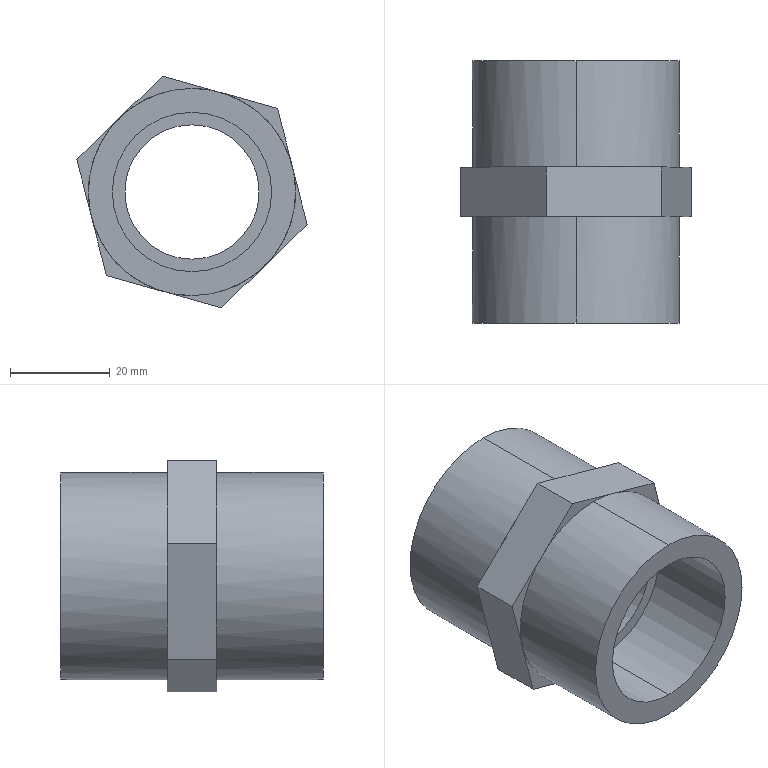Part | SolidWorks | features ICE 3, Revolution 2 | 1 solid | 34 faces | box 46.249 x 52.7 x 46.542 mm | volume 34114 mm3 | plane 22 | cylinder 10 | cone 2 | commonest cylinder face diameters 32 x4 41.6 x4 27 x2
STEP:
#1=CARTESIAN_POINT('',(0.,7.5,-13.5));
#2=VERTEX_POINT('',#1);
#3=CARTESIAN_POINT('',(0.,7.5,13.5));
#4=VERTEX_POINT('',#3);
#5=CARTESIAN_POINT('',(0.,7.5,0.));
#6=DIRECTION('',(0.,1.,0.));
#7=DIRECTION('',(0.,0.,1.));
#8=AXIS2_PLACEMENT_3D('',#5,#6,#7);
#9=CIRCLE('',#8,13.5);
#10=EDGE_CURVE('',#2,#4,#9,.T.);
#11=ORIENTED_EDGE('',*,*,#10,.T.);
#12=CARTESIAN_POINT('',(0.,-7.5,13.5));
#13=VERTEX_POINT('',#12);
#14=CARTESIAN_POINT('',(0.,7.5,13.5));
#15=DIRECTION('',(0.,-1.,0.));
#16=VECTOR('',#15,1000.);
#17=LINE('',#14,#16);
#18=EDGE_CURVE('',#4,#13,#17,.T.);
#19=ORIENTED_EDGE('',*,*,#18,.T.);
#20=CARTESIAN_POINT('',(0.,-7.5,-13.5));
#21=VERTEX_POINT('',#20);
#22=CARTESIAN_POINT('',(0.,-7.5,0.));
#23=DIRECTION('',(0.,1.,0.));
#24=DIRECTION('',(0.,0.,1.));
#25=AXIS2_PLACEMENT_3D('',#22,#23,#24);
#26=CIRCLE('',#25,13.5);
#27=EDGE_CURVE('',#21,#13,#26,.T.);
#28=ORIENTED_EDGE('',*,*,#27,.F.);
#29=CARTESIAN_POINT('',(0.,7.5,-13.5));
#30=DIRECTION('',(0.,-1.,0.));
#31=VECTOR('',#30,1000.);
#32=LINE('',#29,#31);
#33=EDGE_CURVE('',#2,#21,#32,.T.);
#34=ORIENTED_EDGE('',*,*,#33,.F.);
#35=EDGE_LOOP('',(#11,#19,#28,#34));
#36=FACE_OUTER_BOUND('',#35,.T.);
#37=CARTESIAN_POINT('',(0.,7.5,0.));
#38=DIRECTION('',(0.,-1.,0.));
#39=DIRECTION('',(0.,0.,-1.));
#40=AXIS2_PLACEMENT_3D('',#37,#38,#39);
#41=CYLINDRICAL_SURFACE('',#40,13.5);
#42=ADVANCED_FACE('',(#36),#41,.F.);
#43=CARTESIAN_POINT('',(0.,26.2,16.));
#44=VERTEX_POINT('',#43);
#45=CARTESIAN_POINT('',(0.,26.2,-16.));
#46=VERTEX_POINT('',#45);
#47=CARTESIAN_POINT('',(0.,26.2,0.));
#48=DIRECTION('',(0.,-1.,0.));
#49=DIRECTION('',(0.,0.,-1.));
#50=AXIS2_PLACEMENT_3D('',#47,#48,#49);
#51=CIRCLE('',#50,16.);
#52=EDGE_CURVE('',#44,#46,#51,.T.);
#53=ORIENTED_EDGE('',*,*,#52,.T.);
#54=CARTESIAN_POINT('',(0.,26.35,-16.15));
#55=VERTEX_POINT('',#54);
#56=CARTESIAN_POINT('',(0.,26.2,-16.));
#57=DIRECTION('',(0.,0.7071,-0.7071));
#58=VECTOR('',#57,1000.);
#59=LINE('',#56,#58);
#60=EDGE_CURVE('',#46,#55,#59,.T.);
#61=ORIENTED_EDGE('',*,*,#60,.T.);
#62=CARTESIAN_POINT('',(0.,26.35,16.15));
#63=VERTEX_POINT('',#62);
#64=CARTESIAN_POINT('',(0.,26.35,0.));
#65=DIRECTION('',(0.,-1.,0.));
#66=DIRECTION('',(0.,0.,-1.));
#67=AXIS2_PLACEMENT_3D('',#64,#65,#66);
#68=CIRCLE('',#67,16.15);
#69=EDGE_CURVE('',#63,#55,#68,.T.);
#70=ORIENTED_EDGE('',*,*,#69,.F.);
#71=CARTESIAN_POINT('',(0.,26.2,16.));
#72=DIRECTION('',(0.,0.7071,0.7071));
#73=VECTOR('',#72,1000.);
#74=LINE('',#71,#73);
#75=EDGE_CURVE('',#44,#63,#74,.T.);
#76=ORIENTED_EDGE('',*,*,#75,.F.);
#77=EDGE_LOOP('',(#53,#61,#70,#76));
#78=FACE_OUTER_BOUND('',#77,.T.);
#79=CARTESIAN_POINT('',(0.,26.2,0.));
#80=DIRECTION('',(0.,1.,0.));
#81=DIRECTION('',(0.,0.,1.));
#82=AXIS2_PLACEMENT_3D('',#79,#80,#81);
#83=CONICAL_SURFACE('',#82,16.,0.7854);
#84=ADVANCED_FACE('',(#78),#83,.F.);
#85=CARTESIAN_POINT('',(0.,26.35,-20.8));
#86=VERTEX_POINT('',#85);
#87=CARTESIAN_POINT('',(0.,26.35,20.8));
#88=VERTEX_POINT('',#87);
#89=CARTESIAN_POINT('',(0.,26.35,0.));
#90=DIRECTION('',(0.,-1.,0.));
#91=DIRECTION('',(0.,0.,-1.));
#92=AXIS2_PLACEMENT_3D('',#89,#90,#91);
#93=CIRCLE('',#92,20.8);
#94=EDGE_CURVE('',#86,#88,#93,.T.);
#95=ORIENTED_EDGE('',*,*,#94,.T.);
#96=CARTESIAN_POINT('',(0.,5.,20.8));
#97=VERTEX_POINT('',#96);
#98=CARTESIAN_POINT('',(0.,-26.35,20.8));
#99=DIRECTION('',(0.,-1.,0.));
#100=VECTOR('',#99,1000.);
#101=LINE('',#98,#100);
#102=EDGE_CURVE('',#88,#97,#101,.T.);
#103=ORIENTED_EDGE('',*,*,#102,.T.);
#104=CARTESIAN_POINT('',(5.62,5.,20.026));
#105=VERTEX_POINT('',#104);
#106=CARTESIAN_POINT('',(0.,5.,0.));
#107=DIRECTION('',(0.,1.,0.));
#108=DIRECTION('',(0.,0.,1.));
#109=AXIS2_PLACEMENT_3D('',#106,#107,#108);
#110=CIRCLE('',#109,20.8);
#111=EDGE_CURVE('',#97,#105,#110,.T.);
#112=ORIENTED_EDGE('',*,*,#111,.T.);
#113=CARTESIAN_POINT('',(20.153,5.,5.146));
#114=VERTEX_POINT('',#113);
#115=CARTESIAN_POINT('',(0.,5.,0.));
#116=DIRECTION('',(0.,1.,0.));
#117=DIRECTION('',(0.,0.,1.));
#118=AXIS2_PLACEMENT_3D('',#115,#116,#117);
#119=CIRCLE('',#118,20.8);
#120=EDGE_CURVE('',#105,#114,#119,.T.);
#121=ORIENTED_EDGE('',*,*,#120,.T.);
#122=CARTESIAN_POINT('',(14.533,5.,-14.88));
#123=VERTEX_POINT('',#122);
#124=CARTESIAN_POINT('',(0.,5.,0.));
#125=DIRECTION('',(0.,1.,0.));
#126=DIRECTION('',(0.,0.,1.));
#127=AXIS2_PLACEMENT_3D('',#124,#125,#126);
#128=CIRCLE('',#127,20.8);
#129=EDGE_CURVE('',#114,#123,#128,.T.);
#130=ORIENTED_EDGE('',*,*,#129,.T.);
#131=CARTESIAN_POINT('',(0.,5.,-20.8));
#132=VERTEX_POINT('',#131);
#133=CARTESIAN_POINT('',(0.,5.,0.));
#134=DIRECTION('',(0.,1.,0.));
#135=DIRECTION('',(0.,0.,1.));
#136=AXIS2_PLACEMENT_3D('',#133,#134,#135);
#137=CIRCLE('',#136,20.8);
#138=EDGE_CURVE('',#123,#132,#137,.T.);
#139=ORIENTED_EDGE('',*,*,#138,.T.);
#140=CARTESIAN_POINT('',(0.,-26.35,-20.8));
#141=DIRECTION('',(0.,-1.,0.));
#142=VECTOR('',#141,1000.);
#143=LINE('',#140,#142);
#144=EDGE_CURVE('',#86,#132,#143,.T.);
#145=ORIENTED_EDGE('',*,*,#144,.F.);
#146=EDGE_LOOP('',(#95,#103,#112,#121,#130,#139,#145));
#147=FACE_OUTER_BOUND('',#146,.T.);
#148=CARTESIAN_POINT('',(0.,-26.35,0.));
#149=DIRECTION('',(0.,-1.,0.));
#150=DIRECTION('',(0.,0.,-1.));
#151=AXIS2_PLACEMENT_3D('',#148,#149,#150);
#152=CYLINDRICAL_SURFACE('',#151,20.8);
#153=ADVANCED_FACE('',(#147),#152,.T.);
#154=ORIENTED_EDGE('',*,*,#52,.F.);
#155=CARTESIAN_POINT('',(0.,7.5,16.));
#156=VERTEX_POINT('',#155);
#157=CARTESIAN_POINT('',(0.,-26.35,16.));
#158=DIRECTION('',(0.,-1.,0.));
#159=VECTOR('',#158,1000.);
#160=LINE('',#157,#159);
#161=EDGE_CURVE('',#44,#156,#160,.T.);
#162=ORIENTED_EDGE('',*,*,#161,.T.);
#163=CARTESIAN_POINT('',(0.,7.5,-16.));
#164=VERTEX_POINT('',#163);
#165=CARTESIAN_POINT('',(0.,7.5,0.));
#166=DIRECTION('',(0.,-1.,0.));
#167=DIRECTION('',(0.,0.,1.));
#168=AXIS2_PLACEMENT_3D('',#165,#166,#167);
#169=CIRCLE('',#168,16.);
#170=EDGE_CURVE('',#156,#164,#169,.T.);
#171=ORIENTED_EDGE('',*,*,#170,.T.);
#172=CARTESIAN_POINT('',(0.,-26.35,-16.));
#173=DIRECTION('',(0.,-1.,0.));
#174=VECTOR('',#173,1000.);
#175=LINE('',#172,#174);
#176=EDGE_CURVE('',#46,#164,#175,.T.);
#177=ORIENTED_EDGE('',*,*,#176,.F.);
#178=EDGE_LOOP('',(#154,#162,#171,#177));
#179=FACE_OUTER_BOUND('',#178,.T.);
#180=CARTESIAN_POINT('',(0.,-26.35,0.));
#181=DIRECTION('',(0.,-1.,0.));
#182=DIRECTION('',(0.,0.,-1.));
#183=AXIS2_PLACEMENT_3D('',#180,#181,#182);
#184=CYLINDRICAL_SURFACE('',#183,16.);
#185=ADVANCED_FACE('',(#179),#184,.F.);
#186=CARTESIAN_POINT('',(0.,-5.,20.8));
#187=VERTEX_POINT('',#186);
#188=CARTESIAN_POINT('',(5.62,-5.,20.026));
#189=VERTEX_POINT('',#188);
#190=CARTESIAN_POINT('',(0.,-5.,0.));
#191=DIRECTION('',(0.,1.,0.));
#192=DIRECTION('',(0.,0.,1.));
#193=AXIS2_PLACEMENT_3D('',#190,#191,#192);
#194=CIRCLE('',#193,20.8);
#195=EDGE_CURVE('',#187,#189,#194,.T.);
#196=ORIENTED_EDGE('',*,*,#195,.F.);
#197=CARTESIAN_POINT('',(0.,-26.35,20.8));
#198=VERTEX_POINT('',#197);
#199=CARTESIAN_POINT('',(0.,-26.35,20.8));
#200=DIRECTION('',(0.,-1.,0.));
#201=VECTOR('',#200,1000.);
#202=LINE('',#199,#201);
#203=EDGE_CURVE('',#187,#198,#202,.T.);
#204=ORIENTED_EDGE('',*,*,#203,.T.);
#205=CARTESIAN_POINT('',(0.,-26.35,-20.8));
#206=VERTEX_POINT('',#205);
#207=CARTESIAN_POINT('',(0.,-26.35,0.));
#208=DIRECTION('',(0.,-1.,0.));
#209=DIRECTION('',(0.,0.,-1.));
#210=AXIS2_PLACEMENT_3D('',#207,#208,#209);
#211=CIRCLE('',#210,20.8);
#212=EDGE_CURVE('',#206,#198,#211,.T.);
#213=ORIENTED_EDGE('',*,*,#212,.F.);
#214=CARTESIAN_POINT('',(0.,-5.,-20.8));
#215=VERTEX_POINT('',#214);
#216=CARTESIAN_POINT('',(0.,-26.35,-20.8));
#217=DIRECTION('',(0.,-1.,0.));
#218=VECTOR('',#217,1000.);
#219=LINE('',#216,#218);
#220=EDGE_CURVE('',#215,#206,#219,.T.);
#221=ORIENTED_EDGE('',*,*,#220,.F.);
#222=CARTESIAN_POINT('',(14.533,-5.,-14.88));
#223=VERTEX_POINT('',#222);
#224=CARTESIAN_POINT('',(0.,-5.,0.));
#225=DIRECTION('',(0.,1.,0.));
#226=DIRECTION('',(0.,0.,1.));
#227=AXIS2_PLACEMENT_3D('',#224,#225,#226);
#228=CIRCLE('',#227,20.8);
#229=EDGE_CURVE('',#223,#215,#228,.T.);
#230=ORIENTED_EDGE('',*,*,#229,.F.);
#231=CARTESIAN_POINT('',(20.153,-5.,5.146));
#232=VERTEX_POINT('',#231);
#233=CARTESIAN_POINT('',(0.,-5.,0.));
#234=DIRECTION('',(0.,1.,0.));
#235=DIRECTION('',(0.,0.,1.));
#236=AXIS2_PLACEMENT_3D('',#233,#234,#235);
#237=CIRCLE('',#236,20.8);
#238=EDGE_CURVE('',#232,#223,#237,.T.);
#239=ORIENTED_EDGE('',*,*,#238,.F.);
#240=CARTESIAN_POINT('',(0.,-5.,0.));
#241=DIRECTION('',(0.,1.,0.));
#242=DIRECTION('',(0.,0.,1.));
#243=AXIS2_PLACEMENT_3D('',#240,#241,#242);
#244=CIRCLE('',#243,20.8);
#245=EDGE_CURVE('',#189,#232,#244,.T.);
#246=ORIENTED_EDGE('',*,*,#245,.F.);
#247=EDGE_LOOP('',(#196,#204,#213,#221,#230,#239,#246));
#248=FACE_OUTER_BOUND('',#247,.T.);
#249=CARTESIAN_POINT('',(0.,-26.35,0.));
#250=DIRECTION('',(0.,-1.,0.));
#251=DIRECTION('',(0.,0.,-1.));
#252=AXIS2_PLACEMENT_3D('',#249,#250,#251);
#253=CYLINDRICAL_SURFACE('',#252,20.8);
#254=ADVANCED_FACE('',(#248),#253,.T.);
#255=CARTESIAN_POINT('',(0.,-7.5,16.));
#256=VERTEX_POINT('',#255);
#257=CARTESIAN_POINT('',(0.,-7.5,-16.));
#258=VERTEX_POINT('',#257);
#259=CARTESIAN_POINT('',(0.,-7.5,0.));
#260=DIRECTION('',(0.,-1.,0.));
#261=DIRECTION('',(0.,0.,1.));
#262=AXIS2_PLACEMENT_3D('',#259,#260,#261);
#263=CIRCLE('',#262,16.);
#264=EDGE_CURVE('',#256,#258,#263,.T.);
#265=ORIENTED_EDGE('',*,*,#264,.F.);
#266=CARTESIAN_POINT('',(0.,-26.35,16.));
#267=VERTEX_POINT('',#266);
#268=CARTESIAN_POINT('',(0.,-26.35,16.));
#269=DIRECTION('',(0.,-1.,0.));
#270=VECTOR('',#269,1000.);
#271=LINE('',#268,#270);
#272=EDGE_CURVE('',#256,#267,#271,.T.);
#273=ORIENTED_EDGE('',*,*,#272,.T.);
#274=CARTESIAN_POINT('',(0.,-26.35,-16.));
#275=VERTEX_POINT('',#274);
#276=CARTESIAN_POINT('',(0.,-26.35,0.));
#277=DIRECTION('',(0.,-1.,0.));
#278=DIRECTION('',(0.,0.,-1.));
#279=AXIS2_PLACEMENT_3D('',#276,#277,#278);
#280=CIRCLE('',#279,16.);
#281=EDGE_CURVE('',#267,#275,#280,.T.);
#282=ORIENTED_EDGE('',*,*,#281,.T.);
#283=CARTESIAN_POINT('',(0.,-26.35,-16.));
#284=DIRECTION('',(0.,-1.,0.));
#285=VECTOR('',#284,1000.);
#286=LINE('',#283,#285);
#287=EDGE_CURVE('',#258,#275,#286,.T.);
#288=ORIENTED_EDGE('',*,*,#287,.F.);
#289=EDGE_LOOP('',(#265,#273,#282,#288));
#290=FACE_OUTER_BOUND('',#289,.T.);
#291=CARTESIAN_POINT('',(0.,-26.35,0.));
#292=DIRECTION('',(0.,-1.,0.));
#293=DIRECTION('',(0.,0.,-1.));
#294=AXIS2_PLACEMENT_3D('',#291,#292,#293);
#295=CYLINDRICAL_SURFACE('',#294,16.);
#296=ADVANCED_FACE('',(#290),#295,.F.);
#297=ORIENTED_EDGE('',*,*,#272,.F.);
#298=CARTESIAN_POINT('',(0.,-7.5,0.));
#299=DIRECTION('',(0.,-1.,0.));
#300=DIRECTION('',(0.,0.,1.));
#301=AXIS2_PLACEMENT_3D('',#298,#299,#300);
#302=CIRCLE('',#301,16.);
#303=EDGE_CURVE('',#258,#256,#302,.T.);
#304=ORIENTED_EDGE('',*,*,#303,.F.);
#305=ORIENTED_EDGE('',*,*,#287,.T.);
#306=CARTESIAN_POINT('',(0.,-26.35,0.));
#307=DIRECTION('',(0.,-1.,0.));
#308=DIRECTION('',(0.,0.,-1.));
#309=AXIS2_PLACEMENT_3D('',#306,#307,#308);
#310=CIRCLE('',#309,16.);
#311=EDGE_CURVE('',#275,#267,#310,.T.);
#312=ORIENTED_EDGE('',*,*,#311,.T.);
#313=EDGE_LOOP('',(#297,#304,#305,#312));
#314=FACE_OUTER_BOUND('',#313,.T.);
#315=CARTESIAN_POINT('',(0.,-26.35,0.));
#316=DIRECTION('',(0.,-1.,0.));
#317=DIRECTION('',(0.,0.,-1.));
#318=AXIS2_PLACEMENT_3D('',#315,#316,#317);
#319=CYLINDRICAL_SURFACE('',#318,16.);
#320=ADVANCED_FACE('',(#314),#319,.F.);
#321=CARTESIAN_POINT('',(23.124,5.,-6.49));
#322=VERTEX_POINT('',#321);
#323=CARTESIAN_POINT('',(17.182,5.,16.781));
#324=DIRECTION('',(0.2474,0.,-0.9689));
#325=VECTOR('',#324,1000.);
#326=LINE('',#323,#325);
#327=EDGE_CURVE('',#114,#322,#326,.T.);
#328=ORIENTED_EDGE('',*,*,#327,.F.);
#329=CARTESIAN_POINT('',(17.182,5.,16.781));
#330=VERTEX_POINT('',#329);
#331=CARTESIAN_POINT('',(17.182,5.,16.781));
#332=DIRECTION('',(0.2474,0.,-0.9689));
#333=VECTOR('',#332,1000.);
#334=LINE('',#331,#333);
#335=EDGE_CURVE('',#330,#114,#334,.T.);
#336=ORIENTED_EDGE('',*,*,#335,.F.);
#337=CARTESIAN_POINT('',(17.182,-5.,16.781));
#338=VERTEX_POINT('',#337);
#339=CARTESIAN_POINT('',(17.182,5.,16.781));
#340=DIRECTION('',(0.,-1.,0.));
#341=VECTOR('',#340,1000.);
#342=LINE('',#339,#341);
#343=EDGE_CURVE('',#330,#338,#342,.T.);
#344=ORIENTED_EDGE('',*,*,#343,.T.);
#345=CARTESIAN_POINT('',(17.182,-5.,16.781));
#346=DIRECTION('',(0.2474,0.,-0.9689));
#347=VECTOR('',#346,1000.);
#348=LINE('',#345,#347);
#349=EDGE_CURVE('',#338,#232,#348,.T.);
#350=ORIENTED_EDGE('',*,*,#349,.T.);
#351=CARTESIAN_POINT('',(23.124,-5.,-6.49));
#352=VERTEX_POINT('',#351);
#353=CARTESIAN_POINT('',(17.182,-5.,16.781));
#354=DIRECTION('',(0.2474,0.,-0.9689));
#355=VECTOR('',#354,1000.);
#356=LINE('',#353,#355);
#357=EDGE_CURVE('',#232,#352,#356,.T.);
#358=ORIENTED_EDGE('',*,*,#357,.T.);
#359=CARTESIAN_POINT('',(23.124,5.,-6.49));
#360=DIRECTION('',(0.,-1.,0.));
#361=VECTOR('',#360,1000.);
#362=LINE('',#359,#361);
#363=EDGE_CURVE('',#322,#352,#362,.T.);
#364=ORIENTED_EDGE('',*,*,#363,.F.);
#365=EDGE_LOOP('',(#328,#336,#344,#350,#358,#364));
#366=FACE_OUTER_BOUND('',#365,.T.);
#367=CARTESIAN_POINT('',(17.182,5.,16.781));
#368=DIRECTION('',(-0.9689,0.,-0.2474));
#369=DIRECTION('',(-0.2474,0.,0.9689));
#370=AXIS2_PLACEMENT_3D('',#367,#368,#369);
#371=PLANE('',#370);
#372=ADVANCED_FACE('',(#366),#371,.F.);
#373=CARTESIAN_POINT('',(5.942,5.,-23.271));
#374=VERTEX_POINT('',#373);
#375=CARTESIAN_POINT('',(23.124,5.,-6.49));
#376=DIRECTION('',(-0.7154,0.,-0.6987));
#377=VECTOR('',#376,1000.);
#378=LINE('',#375,#377);
#379=EDGE_CURVE('',#123,#374,#378,.T.);
#380=ORIENTED_EDGE('',*,*,#379,.F.);
#381=CARTESIAN_POINT('',(23.124,5.,-6.49));
#382=DIRECTION('',(-0.7154,0.,-0.6987));
#383=VECTOR('',#382,1000.);
#384=LINE('',#381,#383);
#385=EDGE_CURVE('',#322,#123,#384,.T.);
#386=ORIENTED_EDGE('',*,*,#385,.F.);
#387=ORIENTED_EDGE('',*,*,#363,.T.);
#388=CARTESIAN_POINT('',(23.124,-5.,-6.49));
#389=DIRECTION('',(-0.7154,0.,-0.6987));
#390=VECTOR('',#389,1000.);
#391=LINE('',#388,#390);
#392=EDGE_CURVE('',#352,#223,#391,.T.);
#393=ORIENTED_EDGE('',*,*,#392,.T.);
#394=CARTESIAN_POINT('',(5.942,-5.,-23.271));
#395=VERTEX_POINT('',#394);
#396=CARTESIAN_POINT('',(23.124,-5.,-6.49));
#397=DIRECTION('',(-0.7154,0.,-0.6987));
#398=VECTOR('',#397,1000.);
#399=LINE('',#396,#398);
#400=EDGE_CURVE('',#223,#395,#399,.T.);
#401=ORIENTED_EDGE('',*,*,#400,.T.);
#402=CARTESIAN_POINT('',(5.942,5.,-23.271));
#403=DIRECTION('',(0.,-1.,0.));
#404=VECTOR('',#403,1000.);
#405=LINE('',#402,#404);
#406=EDGE_CURVE('',#374,#395,#405,.T.);
#407=ORIENTED_EDGE('',*,*,#406,.F.);
#408=EDGE_LOOP('',(#380,#386,#387,#393,#401,#407));
#409=FACE_OUTER_BOUND('',#408,.T.);
#410=CARTESIAN_POINT('',(23.124,5.,-6.49));
#411=DIRECTION('',(-0.6987,0.,0.7154));
#412=DIRECTION('',(0.7154,0.,0.6987));
#413=AXIS2_PLACEMENT_3D('',#410,#411,#412);
#414=PLANE('',#413);
#415=ADVANCED_FACE('',(#409),#414,.F.);
#416=CARTESIAN_POINT('',(-5.62,5.,-20.026));
#417=VERTEX_POINT('',#416);
#418=CARTESIAN_POINT('',(-17.182,5.,-16.781));
#419=VERTEX_POINT('',#418);
#420=CARTESIAN_POINT('',(5.942,5.,-23.271));
#421=DIRECTION('',(-0.9628,0.,0.2702));
#422=VECTOR('',#421,1000.);
#423=LINE('',#420,#422);
#424=EDGE_CURVE('',#417,#419,#423,.T.);
#425=ORIENTED_EDGE('',*,*,#424,.F.);
#426=CARTESIAN_POINT('',(5.942,5.,-23.271));
#427=DIRECTION('',(-0.9628,0.,0.2702));
#428=VECTOR('',#427,1000.);
#429=LINE('',#426,#428);
#430=EDGE_CURVE('',#374,#417,#429,.T.);
#431=ORIENTED_EDGE('',*,*,#430,.F.);
#432=ORIENTED_EDGE('',*,*,#406,.T.);
#433=CARTESIAN_POINT('',(-5.62,-5.,-20.026));
#434=VERTEX_POINT('',#433);
#435=CARTESIAN_POINT('',(5.942,-5.,-23.271));
#436=DIRECTION('',(-0.9628,0.,0.2702));
#437=VECTOR('',#436,1000.);
#438=LINE('',#435,#437);
#439=EDGE_CURVE('',#395,#434,#438,.T.);
#440=ORIENTED_EDGE('',*,*,#439,.T.);
#441=CARTESIAN_POINT('',(-17.182,-5.,-16.781));
#442=VERTEX_POINT('',#441);
#443=CARTESIAN_POINT('',(5.942,-5.,-23.271));
#444=DIRECTION('',(-0.9628,0.,0.2702));
#445=VECTOR('',#444,1000.);
#446=LINE('',#443,#445);
#447=EDGE_CURVE('',#434,#442,#446,.T.);
#448=ORIENTED_EDGE('',*,*,#447,.T.);
#449=CARTESIAN_POINT('',(-17.182,5.,-16.781));
#450=DIRECTION('',(0.,-1.,0.));
#451=VECTOR('',#450,1000.);
#452=LINE('',#449,#451);
#453=EDGE_CURVE('',#419,#442,#452,.T.);
#454=ORIENTED_EDGE('',*,*,#453,.F.);
#455=EDGE_LOOP('',(#425,#431,#432,#440,#448,#454));
#456=FACE_OUTER_BOUND('',#455,.T.);
#457=CARTESIAN_POINT('',(5.942,5.,-23.271));
#458=DIRECTION('',(0.2702,0.,0.9628));
#459=DIRECTION('',(0.9628,0.,-0.2702));
#460=AXIS2_PLACEMENT_3D('',#457,#458,#459);
#461=PLANE('',#460);
#462=ADVANCED_FACE('',(#456),#461,.F.);
#463=CARTESIAN_POINT('',(-20.153,5.,-5.146));
#464=VERTEX_POINT('',#463);
#465=CARTESIAN_POINT('',(-23.124,5.,6.49));
#466=VERTEX_POINT('',#465);
#467=CARTESIAN_POINT('',(-17.182,5.,-16.781));
#468=DIRECTION('',(-0.2474,0.,0.9689));
#469=VECTOR('',#468,1000.);
#470=LINE('',#467,#469);
#471=EDGE_CURVE('',#464,#466,#470,.T.);
#472=ORIENTED_EDGE('',*,*,#471,.F.);
#473=CARTESIAN_POINT('',(-17.182,5.,-16.781));
#474=DIRECTION('',(-0.2474,0.,0.9689));
#475=VECTOR('',#474,1000.);
#476=LINE('',#473,#475);
#477=EDGE_CURVE('',#419,#464,#476,.T.);
#478=ORIENTED_EDGE('',*,*,#477,.F.);
#479=ORIENTED_EDGE('',*,*,#453,.T.);
#480=CARTESIAN_POINT('',(-20.153,-5.,-5.146));
#481=VERTEX_POINT('',#480);
#482=CARTESIAN_POINT('',(-17.182,-5.,-16.781));
#483=DIRECTION('',(-0.2474,0.,0.9689));
#484=VECTOR('',#483,1000.);
#485=LINE('',#482,#484);
#486=EDGE_CURVE('',#442,#481,#485,.T.);
#487=ORIENTED_EDGE('',*,*,#486,.T.);
#488=CARTESIAN_POINT('',(-23.124,-5.,6.49));
#489=VERTEX_POINT('',#488);
#490=CARTESIAN_POINT('',(-17.182,-5.,-16.781));
#491=DIRECTION('',(-0.2474,0.,0.9689));
#492=VECTOR('',#491,1000.);
#493=LINE('',#490,#492);
#494=EDGE_CURVE('',#481,#489,#493,.T.);
#495=ORIENTED_EDGE('',*,*,#494,.T.);
#496=CARTESIAN_POINT('',(-23.124,5.,6.49));
#497=DIRECTION('',(0.,-1.,0.));
#498=VECTOR('',#497,1000.);
#499=LINE('',#496,#498);
#500=EDGE_CURVE('',#466,#489,#499,.T.);
#501=ORIENTED_EDGE('',*,*,#500,.F.);
#502=EDGE_LOOP('',(#472,#478,#479,#487,#495,#501));
#503=FACE_OUTER_BOUND('',#502,.T.);
#504=CARTESIAN_POINT('',(-17.182,5.,-16.781));
#505=DIRECTION('',(0.9689,0.,0.2474));
#506=DIRECTION('',(0.2474,0.,-0.9689));
#507=AXIS2_PLACEMENT_3D('',#504,#505,#506);
#508=PLANE('',#507);
#509=ADVANCED_FACE('',(#503),#508,.F.);
#510=CARTESIAN_POINT('',(-14.533,5.,14.88));
#511=VERTEX_POINT('',#510);
#512=CARTESIAN_POINT('',(-5.942,5.,23.271));
#513=VERTEX_POINT('',#512);
#514=CARTESIAN_POINT('',(-23.124,5.,6.49));
#515=DIRECTION('',(0.7154,0.,0.6987));
#516=VECTOR('',#515,1000.);
#517=LINE('',#514,#516);
#518=EDGE_CURVE('',#511,#513,#517,.T.);
#519=ORIENTED_EDGE('',*,*,#518,.F.);
#520=CARTESIAN_POINT('',(-23.124,5.,6.49));
#521=DIRECTION('',(0.7154,0.,0.6987));
#522=VECTOR('',#521,1000.);
#523=LINE('',#520,#522);
#524=EDGE_CURVE('',#466,#511,#523,.T.);
#525=ORIENTED_EDGE('',*,*,#524,.F.);
#526=ORIENTED_EDGE('',*,*,#500,.T.);
#527=CARTESIAN_POINT('',(-14.533,-5.,14.88));
#528=VERTEX_POINT('',#527);
#529=CARTESIAN_POINT('',(-23.124,-5.,6.49));
#530=DIRECTION('',(0.7154,0.,0.6987));
#531=VECTOR('',#530,1000.);
#532=LINE('',#529,#531);
#533=EDGE_CURVE('',#489,#528,#532,.T.);
#534=ORIENTED_EDGE('',*,*,#533,.T.);
#535=CARTESIAN_POINT('',(-5.942,-5.,23.271));
#536=VERTEX_POINT('',#535);
#537=CARTESIAN_POINT('',(-23.124,-5.,6.49));
#538=DIRECTION('',(0.7154,0.,0.6987));
#539=VECTOR('',#538,1000.);
#540=LINE('',#537,#539);
#541=EDGE_CURVE('',#528,#536,#540,.T.);
#542=ORIENTED_EDGE('',*,*,#541,.T.);
#543=CARTESIAN_POINT('',(-5.942,5.,23.271));
#544=DIRECTION('',(0.,-1.,0.));
#545=VECTOR('',#544,1000.);
#546=LINE('',#543,#545);
#547=EDGE_CURVE('',#513,#536,#546,.T.);
#548=ORIENTED_EDGE('',*,*,#547,.F.);
#549=EDGE_LOOP('',(#519,#525,#526,#534,#542,#548));
#550=FACE_OUTER_BOUND('',#549,.T.);
#551=CARTESIAN_POINT('',(-23.124,5.,6.49));
#552=DIRECTION('',(0.6987,0.,-0.7154));
#553=DIRECTION('',(-0.7154,0.,-0.6987));
#554=AXIS2_PLACEMENT_3D('',#551,#552,#553);
#555=PLANE('',#554);
#556=ADVANCED_FACE('',(#550),#555,.F.);
#557=CARTESIAN_POINT('',(-5.942,5.,23.271));
#558=DIRECTION('',(0.9628,0.,-0.2702));
#559=VECTOR('',#558,1000.);
#560=LINE('',#557,#559);
#561=EDGE_CURVE('',#105,#330,#560,.T.);
#562=ORIENTED_EDGE('',*,*,#561,.F.);
#563=CARTESIAN_POINT('',(-5.942,5.,23.271));
#564=DIRECTION('',(0.9628,0.,-0.2702));
#565=VECTOR('',#564,1000.);
#566=LINE('',#563,#565);
#567=EDGE_CURVE('',#513,#105,#566,.T.);
#568=ORIENTED_EDGE('',*,*,#567,.F.);
#569=ORIENTED_EDGE('',*,*,#547,.T.);
#570=CARTESIAN_POINT('',(-5.942,-5.,23.271));
#571=DIRECTION('',(0.9628,0.,-0.2702));
#572=VECTOR('',#571,1000.);
#573=LINE('',#570,#572);
#574=EDGE_CURVE('',#536,#189,#573,.T.);
#575=ORIENTED_EDGE('',*,*,#574,.T.);
#576=CARTESIAN_POINT('',(-5.942,-5.,23.271));
#577=DIRECTION('',(0.9628,0.,-0.2702));
#578=VECTOR('',#577,1000.);
#579=LINE('',#576,#578);
#580=EDGE_CURVE('',#189,#338,#579,.T.);
#581=ORIENTED_EDGE('',*,*,#580,.T.);
#582=ORIENTED_EDGE('',*,*,#343,.F.);
#583=EDGE_LOOP('',(#562,#568,#569,#575,#581,#582));
#584=FACE_OUTER_BOUND('',#583,.T.);
#585=CARTESIAN_POINT('',(-5.942,5.,23.271));
#586=DIRECTION('',(-0.2702,0.,-0.9628));
#587=DIRECTION('',(-0.9628,0.,0.2702));
#588=AXIS2_PLACEMENT_3D('',#585,#586,#587);
#589=PLANE('',#588);
#590=ADVANCED_FACE('',(#584),#589,.F.);
#591=ORIENTED_EDGE('',*,*,#120,.F.);
#592=ORIENTED_EDGE('',*,*,#561,.T.);
#593=ORIENTED_EDGE('',*,*,#335,.T.);
#594=EDGE_LOOP('',(#591,#592,#593));
#595=FACE_OUTER_BOUND('',#594,.T.);
#596=CARTESIAN_POINT('',(0.,5.,0.));
#597=DIRECTION('',(0.,1.,0.));
#598=DIRECTION('',(0.,0.,1.));
#599=AXIS2_PLACEMENT_3D('',#596,#597,#598);
#600=PLANE('',#599);
#601=ADVANCED_FACE('',(#595),#600,.T.);
#602=ORIENTED_EDGE('',*,*,#129,.F.);
#603=ORIENTED_EDGE('',*,*,#327,.T.);
#604=ORIENTED_EDGE('',*,*,#385,.T.);
#605=EDGE_LOOP('',(#602,#603,#604));
#606=FACE_OUTER_BOUND('',#605,.T.);
#607=CARTESIAN_POINT('',(0.,5.,0.));
#608=DIRECTION('',(0.,1.,0.));
#609=DIRECTION('',(0.,0.,1.));
#610=AXIS2_PLACEMENT_3D('',#607,#608,#609);
#611=PLANE('',#610);
#612=ADVANCED_FACE('',(#606),#611,.T.);
#613=ORIENTED_EDGE('',*,*,#138,.F.);
#614=ORIENTED_EDGE('',*,*,#379,.T.);
#615=ORIENTED_EDGE('',*,*,#430,.T.);
#616=CARTESIAN_POINT('',(0.,5.,0.));
#617=DIRECTION('',(0.,1.,0.));
#618=DIRECTION('',(0.,0.,1.));
#619=AXIS2_PLACEMENT_3D('',#616,#617,#618);
#620=CIRCLE('',#619,20.8);
#621=EDGE_CURVE('',#132,#417,#620,.T.);
#622=ORIENTED_EDGE('',*,*,#621,.F.);
#623=EDGE_LOOP('',(#613,#614,#615,#622));
#624=FACE_OUTER_BOUND('',#623,.T.);
#625=CARTESIAN_POINT('',(0.,5.,0.));
#626=DIRECTION('',(0.,1.,0.));
#627=DIRECTION('',(0.,0.,1.));
#628=AXIS2_PLACEMENT_3D('',#625,#626,#627);
#629=PLANE('',#628);
#630=ADVANCED_FACE('',(#624),#629,.T.);
#631=CARTESIAN_POINT('',(0.,5.,0.));
#632=DIRECTION('',(0.,1.,0.));
#633=DIRECTION('',(0.,0.,1.));
#634=AXIS2_PLACEMENT_3D('',#631,#632,#633);
#635=CIRCLE('',#634,20.8);
#636=EDGE_CURVE('',#417,#464,#635,.T.);
#637=ORIENTED_EDGE('',*,*,#636,.F.);
#638=ORIENTED_EDGE('',*,*,#424,.T.);
#639=ORIENTED_EDGE('',*,*,#477,.T.);
#640=EDGE_LOOP('',(#637,#638,#639));
#641=FACE_OUTER_BOUND('',#640,.T.);
#642=CARTESIAN_POINT('',(0.,5.,0.));
#643=DIRECTION('',(0.,1.,0.));
#644=DIRECTION('',(0.,0.,1.));
#645=AXIS2_PLACEMENT_3D('',#642,#643,#644);
#646=PLANE('',#645);
#647=ADVANCED_FACE('',(#641),#646,.T.);
#648=CARTESIAN_POINT('',(0.,5.,0.));
#649=DIRECTION('',(0.,1.,0.));
#650=DIRECTION('',(0.,0.,1.));
#651=AXIS2_PLACEMENT_3D('',#648,#649,#650);
#652=CIRCLE('',#651,20.8);
#653=EDGE_CURVE('',#464,#511,#652,.T.);
#654=ORIENTED_EDGE('',*,*,#653,.F.);
#655=ORIENTED_EDGE('',*,*,#471,.T.);
#656=ORIENTED_EDGE('',*,*,#524,.T.);
#657=EDGE_LOOP('',(#654,#655,#656));
#658=FACE_OUTER_BOUND('',#657,.T.);
#659=CARTESIAN_POINT('',(0.,5.,0.));
#660=DIRECTION('',(0.,1.,0.));
#661=DIRECTION('',(0.,0.,1.));
#662=AXIS2_PLACEMENT_3D('',#659,#660,#661);
#663=PLANE('',#662);
#664=ADVANCED_FACE('',(#658),#663,.T.);
#665=ORIENTED_EDGE('',*,*,#580,.F.);
#666=ORIENTED_EDGE('',*,*,#245,.T.);
#667=ORIENTED_EDGE('',*,*,#349,.F.);
#668=EDGE_LOOP('',(#665,#666,#667));
#669=FACE_OUTER_BOUND('',#668,.T.);
#670=CARTESIAN_POINT('',(0.,-5.,0.));
#671=DIRECTION('',(0.,1.,0.));
#672=DIRECTION('',(0.,0.,1.));
#673=AXIS2_PLACEMENT_3D('',#670,#671,#672);
#674=PLANE('',#673);
#675=ADVANCED_FACE('',(#669),#674,.F.);
#676=ORIENTED_EDGE('',*,*,#357,.F.);
#677=ORIENTED_EDGE('',*,*,#238,.T.);
#678=ORIENTED_EDGE('',*,*,#392,.F.);
#679=EDGE_LOOP('',(#676,#677,#678));
#680=FACE_OUTER_BOUND('',#679,.T.);
#681=CARTESIAN_POINT('',(0.,-5.,0.));
#682=DIRECTION('',(0.,1.,0.));
#683=DIRECTION('',(0.,0.,1.));
#684=AXIS2_PLACEMENT_3D('',#681,#682,#683);
#685=PLANE('',#684);
#686=ADVANCED_FACE('',(#680),#685,.F.);
#687=ORIENTED_EDGE('',*,*,#400,.F.);
#688=ORIENTED_EDGE('',*,*,#229,.T.);
#689=CARTESIAN_POINT('',(0.,-5.,0.));
#690=DIRECTION('',(0.,1.,0.));
#691=DIRECTION('',(0.,0.,1.));
#692=AXIS2_PLACEMENT_3D('',#689,#690,#691);
#693=CIRCLE('',#692,20.8);
#694=EDGE_CURVE('',#215,#434,#693,.T.);
#695=ORIENTED_EDGE('',*,*,#694,.T.);
#696=ORIENTED_EDGE('',*,*,#439,.F.);
#697=EDGE_LOOP('',(#687,#688,#695,#696));
#698=FACE_OUTER_BOUND('',#697,.T.);
#699=CARTESIAN_POINT('',(0.,-5.,0.));
#700=DIRECTION('',(0.,1.,0.));
#701=DIRECTION('',(0.,0.,1.));
#702=AXIS2_PLACEMENT_3D('',#699,#700,#701);
#703=PLANE('',#702);
#704=ADVANCED_FACE('',(#698),#703,.F.);
#705=ORIENTED_EDGE('',*,*,#447,.F.);
#706=CARTESIAN_POINT('',(0.,-5.,0.));
#707=DIRECTION('',(0.,1.,0.));
#708=DIRECTION('',(0.,0.,1.));
#709=AXIS2_PLACEMENT_3D('',#706,#707,#708);
#710=CIRCLE('',#709,20.8);
#711=EDGE_CURVE('',#434,#481,#710,.T.);
#712=ORIENTED_EDGE('',*,*,#711,.T.);
#713=ORIENTED_EDGE('',*,*,#486,.F.);
#714=EDGE_LOOP('',(#705,#712,#713));
#715=FACE_OUTER_BOUND('',#714,.T.);
#716=CARTESIAN_POINT('',(0.,-5.,0.));
#717=DIRECTION('',(0.,1.,0.));
#718=DIRECTION('',(0.,0.,1.));
#719=AXIS2_PLACEMENT_3D('',#716,#717,#718);
#720=PLANE('',#719);
#721=ADVANCED_FACE('',(#715),#720,.F.);
#722=ORIENTED_EDGE('',*,*,#494,.F.);
#723=CARTESIAN_POINT('',(0.,-5.,0.));
#724=DIRECTION('',(0.,1.,0.));
#725=DIRECTION('',(0.,0.,1.));
#726=AXIS2_PLACEMENT_3D('',#723,#724,#725);
#727=CIRCLE('',#726,20.8);
#728=EDGE_CURVE('',#481,#528,#727,.T.);
#729=ORIENTED_EDGE('',*,*,#728,.T.);
#730=ORIENTED_EDGE('',*,*,#533,.F.);
#731=EDGE_LOOP('',(#722,#729,#730));
#732=FACE_OUTER_BOUND('',#731,.T.);
#733=CARTESIAN_POINT('',(0.,-5.,0.));
#734=DIRECTION('',(0.,1.,0.));
#735=DIRECTION('',(0.,0.,1.));
#736=AXIS2_PLACEMENT_3D('',#733,#734,#735);
#737=PLANE('',#736);
#738=ADVANCED_FACE('',(#732),#737,.F.);
#739=CARTESIAN_POINT('',(0.,5.,0.));
#740=DIRECTION('',(0.,1.,0.));
#741=DIRECTION('',(0.,0.,1.));
#742=AXIS2_PLACEMENT_3D('',#739,#740,#741);
#743=CIRCLE('',#742,20.8);
#744=EDGE_CURVE('',#511,#97,#743,.T.);
#745=ORIENTED_EDGE('',*,*,#744,.F.);
#746=ORIENTED_EDGE('',*,*,#518,.T.);
#747=ORIENTED_EDGE('',*,*,#567,.T.);
#748=ORIENTED_EDGE('',*,*,#111,.F.);
#749=EDGE_LOOP('',(#745,#746,#747,#748));
#750=FACE_OUTER_BOUND('',#749,.T.);
#751=CARTESIAN_POINT('',(0.,5.,0.));
#752=DIRECTION('',(0.,1.,0.));
#753=DIRECTION('',(0.,0.,1.));
#754=AXIS2_PLACEMENT_3D('',#751,#752,#753);
#755=PLANE('',#754);
#756=ADVANCED_FACE('',(#750),#755,.T.);
#757=ORIENTED_EDGE('',*,*,#541,.F.);
#758=CARTESIAN_POINT('',(0.,-5.,0.));
#759=DIRECTION('',(0.,1.,0.));
#760=DIRECTION('',(0.,0.,1.));
#761=AXIS2_PLACEMENT_3D('',#758,#759,#760);
#762=CIRCLE('',#761,20.8);
#763=EDGE_CURVE('',#528,#187,#762,.T.);
#764=ORIENTED_EDGE('',*,*,#763,.T.);
#765=ORIENTED_EDGE('',*,*,#195,.T.);
#766=ORIENTED_EDGE('',*,*,#574,.F.);
#767=EDGE_LOOP('',(#757,#764,#765,#766));
#768=FACE_OUTER_BOUND('',#767,.T.);
#769=CARTESIAN_POINT('',(0.,-5.,0.));
#770=DIRECTION('',(0.,1.,0.));
#771=DIRECTION('',(0.,0.,1.));
#772=AXIS2_PLACEMENT_3D('',#769,#770,#771);
#773=PLANE('',#772);
#774=ADVANCED_FACE('',(#768),#773,.F.);
#775=ORIENTED_EDGE('',*,*,#311,.F.);
#776=ORIENTED_EDGE('',*,*,#281,.F.);
#777=EDGE_LOOP('',(#775,#776));
#778=FACE_BOUND('',#777,.T.);
#779=ORIENTED_EDGE('',*,*,#212,.T.);
#780=CARTESIAN_POINT('',(0.,-26.35,0.));
#781=DIRECTION('',(0.,-1.,0.));
#782=DIRECTION('',(0.,0.,-1.));
#783=AXIS2_PLACEMENT_3D('',#780,#781,#782);
#784=CIRCLE('',#783,20.8);
#785=EDGE_CURVE('',#198,#206,#784,.T.);
#786=ORIENTED_EDGE('',*,*,#785,.T.);
#787=EDGE_LOOP('',(#779,#786));
#788=FACE_OUTER_BOUND('',#787,.T.);
#789=CARTESIAN_POINT('',(-20.8,-26.35,0.));
#790=DIRECTION('',(0.,1.,0.));
#791=DIRECTION('',(0.,0.,1.));
#792=AXIS2_PLACEMENT_3D('',#789,#790,#791);
#793=PLANE('',#792);
#794=ADVANCED_FACE('',(#778,#788),#793,.F.);
#795=ORIENTED_EDGE('',*,*,#203,.F.);
#796=ORIENTED_EDGE('',*,*,#763,.F.);
#797=ORIENTED_EDGE('',*,*,#728,.F.);
#798=ORIENTED_EDGE('',*,*,#711,.F.);
#799=ORIENTED_EDGE('',*,*,#694,.F.);
#800=ORIENTED_EDGE('',*,*,#220,.T.);
#801=ORIENTED_EDGE('',*,*,#785,.F.);
#802=EDGE_LOOP('',(#795,#796,#797,#798,#799,#800,#801));
#803=FACE_OUTER_BOUND('',#802,.T.);
#804=CARTESIAN_POINT('',(0.,-26.35,0.));
#805=DIRECTION('',(0.,-1.,0.));
#806=DIRECTION('',(0.,0.,-1.));
#807=AXIS2_PLACEMENT_3D('',#804,#805,#806);
#808=CYLINDRICAL_SURFACE('',#807,20.8);
#809=ADVANCED_FACE('',(#803),#808,.T.);
#810=ORIENTED_EDGE('',*,*,#161,.F.);
#811=CARTESIAN_POINT('',(0.,26.2,0.));
#812=DIRECTION('',(0.,-1.,0.));
#813=DIRECTION('',(0.,0.,-1.));
#814=AXIS2_PLACEMENT_3D('',#811,#812,#813);
#815=CIRCLE('',#814,16.);
#816=EDGE_CURVE('',#46,#44,#815,.T.);
#817=ORIENTED_EDGE('',*,*,#816,.F.);
#818=ORIENTED_EDGE('',*,*,#176,.T.);
#819=CARTESIAN_POINT('',(0.,7.5,0.));
#820=DIRECTION('',(0.,-1.,0.));
#821=DIRECTION('',(0.,0.,1.));
#822=AXIS2_PLACEMENT_3D('',#819,#820,#821);
#823=CIRCLE('',#822,16.);
#824=EDGE_CURVE('',#164,#156,#823,.T.);
#825=ORIENTED_EDGE('',*,*,#824,.T.);
#826=EDGE_LOOP('',(#810,#817,#818,#825));
#827=FACE_OUTER_BOUND('',#826,.T.);
#828=CARTESIAN_POINT('',(0.,-26.35,0.));
#829=DIRECTION('',(0.,-1.,0.));
#830=DIRECTION('',(0.,0.,-1.));
#831=AXIS2_PLACEMENT_3D('',#828,#829,#830);
#832=CYLINDRICAL_SURFACE('',#831,16.);
#833=ADVANCED_FACE('',(#827),#832,.F.);
#834=ORIENTED_EDGE('',*,*,#102,.F.);
#835=CARTESIAN_POINT('',(0.,26.35,0.));
#836=DIRECTION('',(0.,-1.,0.));
#837=DIRECTION('',(0.,0.,-1.));
#838=AXIS2_PLACEMENT_3D('',#835,#836,#837);
#839=CIRCLE('',#838,20.8);
#840=EDGE_CURVE('',#88,#86,#839,.T.);
#841=ORIENTED_EDGE('',*,*,#840,.T.);
#842=ORIENTED_EDGE('',*,*,#144,.T.);
#843=ORIENTED_EDGE('',*,*,#621,.T.);
#844=ORIENTED_EDGE('',*,*,#636,.T.);
#845=ORIENTED_EDGE('',*,*,#653,.T.);
#846=ORIENTED_EDGE('',*,*,#744,.T.);
#847=EDGE_LOOP('',(#834,#841,#842,#843,#844,#845,#846));
#848=FACE_OUTER_BOUND('',#847,.T.);
#849=CARTESIAN_POINT('',(0.,-26.35,0.));
#850=DIRECTION('',(0.,-1.,0.));
#851=DIRECTION('',(0.,0.,-1.));
#852=AXIS2_PLACEMENT_3D('',#849,#850,#851);
#853=CYLINDRICAL_SURFACE('',#852,20.8);
#854=ADVANCED_FACE('',(#848),#853,.T.);
#855=ORIENTED_EDGE('',*,*,#94,.F.);
#856=ORIENTED_EDGE('',*,*,#840,.F.);
#857=EDGE_LOOP('',(#855,#856));
#858=FACE_OUTER_BOUND('',#857,.T.);
#859=ORIENTED_EDGE('',*,*,#69,.T.);
#860=CARTESIAN_POINT('',(0.,26.35,0.));
#861=DIRECTION('',(0.,-1.,0.));
#862=DIRECTION('',(0.,0.,-1.));
#863=AXIS2_PLACEMENT_3D('',#860,#861,#862);
#864=CIRCLE('',#863,16.15);
#865=EDGE_CURVE('',#55,#63,#864,.T.);
#866=ORIENTED_EDGE('',*,*,#865,.T.);
#867=EDGE_LOOP('',(#859,#866));
#868=FACE_BOUND('',#867,.T.);
#869=CARTESIAN_POINT('',(-16.15,26.35,0.));
#870=DIRECTION('',(0.,-1.,0.));
#871=DIRECTION('',(0.,0.,-1.));
#872=AXIS2_PLACEMENT_3D('',#869,#870,#871);
#873=PLANE('',#872);
#874=ADVANCED_FACE('',(#858,#868),#873,.F.);
#875=ORIENTED_EDGE('',*,*,#60,.F.);
#876=ORIENTED_EDGE('',*,*,#816,.T.);
#877=ORIENTED_EDGE('',*,*,#75,.T.);
#878=ORIENTED_EDGE('',*,*,#865,.F.);
#879=EDGE_LOOP('',(#875,#876,#877,#878));
#880=FACE_OUTER_BOUND('',#879,.T.);
#881=CARTESIAN_POINT('',(0.,26.2,0.));
#882=DIRECTION('',(0.,1.,0.));
#883=DIRECTION('',(0.,0.,1.));
#884=AXIS2_PLACEMENT_3D('',#881,#882,#883);
#885=CONICAL_SURFACE('',#884,16.,0.7854);
#886=ADVANCED_FACE('',(#880),#885,.F.);
#887=ORIENTED_EDGE('',*,*,#10,.F.);
#888=CARTESIAN_POINT('',(0.,7.5,0.));
#889=DIRECTION('',(0.,1.,0.));
#890=DIRECTION('',(0.,0.,1.));
#891=AXIS2_PLACEMENT_3D('',#888,#889,#890);
#892=CIRCLE('',#891,13.5);
#893=EDGE_CURVE('',#4,#2,#892,.T.);
#894=ORIENTED_EDGE('',*,*,#893,.F.);
#895=EDGE_LOOP('',(#887,#894));
#896=FACE_BOUND('',#895,.T.);
#897=ORIENTED_EDGE('',*,*,#824,.F.);
#898=ORIENTED_EDGE('',*,*,#170,.F.);
#899=EDGE_LOOP('',(#897,#898));
#900=FACE_OUTER_BOUND('',#899,.T.);
#901=CARTESIAN_POINT('',(0.,7.5,0.));
#902=DIRECTION('',(0.,1.,0.));
#903=DIRECTION('',(0.,0.,1.));
#904=AXIS2_PLACEMENT_3D('',#901,#902,#903);
#905=PLANE('',#904);
#906=ADVANCED_FACE('',(#896,#900),#905,.T.);
#907=ORIENTED_EDGE('',*,*,#27,.T.);
#908=CARTESIAN_POINT('',(0.,-7.5,0.));
#909=DIRECTION('',(0.,1.,0.));
#910=DIRECTION('',(0.,0.,1.));
#911=AXIS2_PLACEMENT_3D('',#908,#909,#910);
#912=CIRCLE('',#911,13.5);
#913=EDGE_CURVE('',#13,#21,#912,.T.);
#914=ORIENTED_EDGE('',*,*,#913,.T.);
#915=EDGE_LOOP('',(#907,#914));
#916=FACE_BOUND('',#915,.T.);
#917=ORIENTED_EDGE('',*,*,#303,.T.);
#918=ORIENTED_EDGE('',*,*,#264,.T.);
#919=EDGE_LOOP('',(#917,#918));
#920=FACE_OUTER_BOUND('',#919,.T.);
#921=CARTESIAN_POINT('',(0.,-7.5,0.));
#922=DIRECTION('',(0.,1.,0.));
#923=DIRECTION('',(0.,0.,1.));
#924=AXIS2_PLACEMENT_3D('',#921,#922,#923);
#925=PLANE('',#924);
#926=ADVANCED_FACE('',(#916,#920),#925,.F.);
#927=ORIENTED_EDGE('',*,*,#18,.F.);
#928=ORIENTED_EDGE('',*,*,#893,.T.);
#929=ORIENTED_EDGE('',*,*,#33,.T.);
#930=ORIENTED_EDGE('',*,*,#913,.F.);
#931=EDGE_LOOP('',(#927,#928,#929,#930));
#932=FACE_OUTER_BOUND('',#931,.T.);
#933=CARTESIAN_POINT('',(0.,7.5,0.));
#934=DIRECTION('',(0.,-1.,0.));
#935=DIRECTION('',(0.,0.,-1.));
#936=AXIS2_PLACEMENT_3D('',#933,#934,#935);
#937=CYLINDRICAL_SURFACE('',#936,13.5);
#938=ADVANCED_FACE('',(#932),#937,.F.);
#939=CLOSED_SHELL('',(#42,#84,#153,#185,#254,#296,#320,#372,#415,#462,#509,#556,#590,#601,#612,#630,#647,#664,#675,#686,#704,#721,#738,#756,#774,#794,#809,#833,#854,#874,#886,#906,#926,#938));
#940=MANIFOLD_SOLID_BREP('',#939);
#941=CARTESIAN_POINT('',(0.,0.,0.));
#942=DIRECTION('',(0.,0.,1.));
#943=DIRECTION('',(1.,0.,0.));
#944=AXIS2_PLACEMENT_3D('',#941,#942,#943);
#945=(LENGTH_UNIT()NAMED_UNIT(*)SI_UNIT(.MILLI.,.METRE.));
#946=UNCERTAINTY_MEASURE_WITH_UNIT(LENGTH_MEASURE(0.00001),#945,'','');
#947=(NAMED_UNIT(*)PLANE_ANGLE_UNIT()SI_UNIT($,.RADIAN.));
#948=(NAMED_UNIT(*)SI_UNIT($,.STERADIAN.)SOLID_ANGLE_UNIT());
#949=(GEOMETRIC_REPRESENTATION_CONTEXT(3)GLOBAL_UNCERTAINTY_ASSIGNED_CONTEXT((#946))GLOBAL_UNIT_ASSIGNED_CONTEXT((#945,#947,#948))REPRESENTATION_CONTEXT('',''));
#950=ADVANCED_BREP_SHAPE_REPRESENTATION('',(#940,#944),#949);